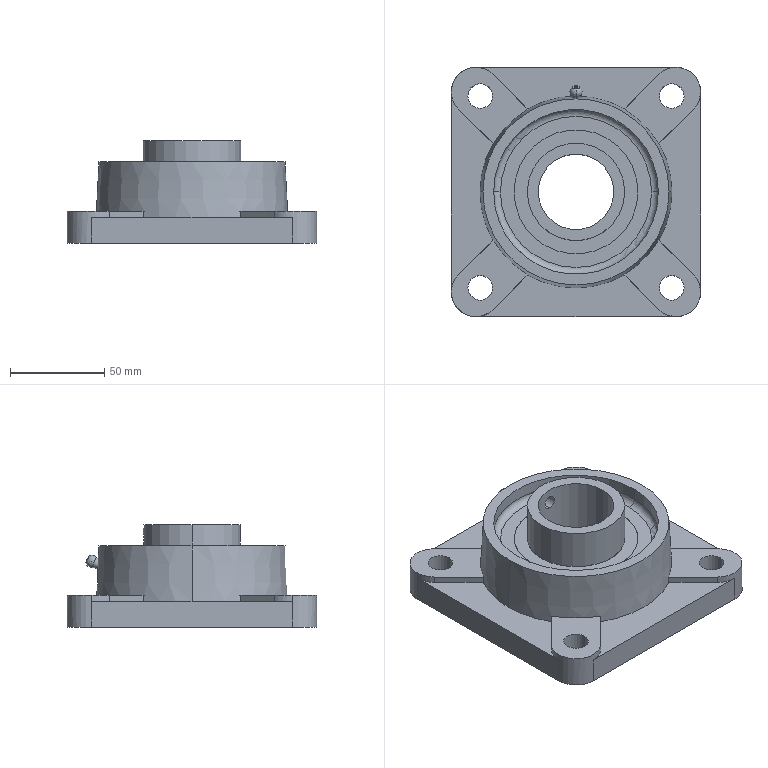Part | SolidWorks | features Revolution 5, Boss 2, RevCut 2, CirPattern 1, Cut 1, Extrusion 1 | 1 solid | 118 faces | box 132 x 132 x 54.2 mm | volume 283670 mm3 | cylinder 58 | plane 42 | sphere 10 | torus 6 | cone 2 | commonest cylinder face diameters 6 x14 26 x12 13 x8 51.6 x6 65.6 x6 87.2 x4